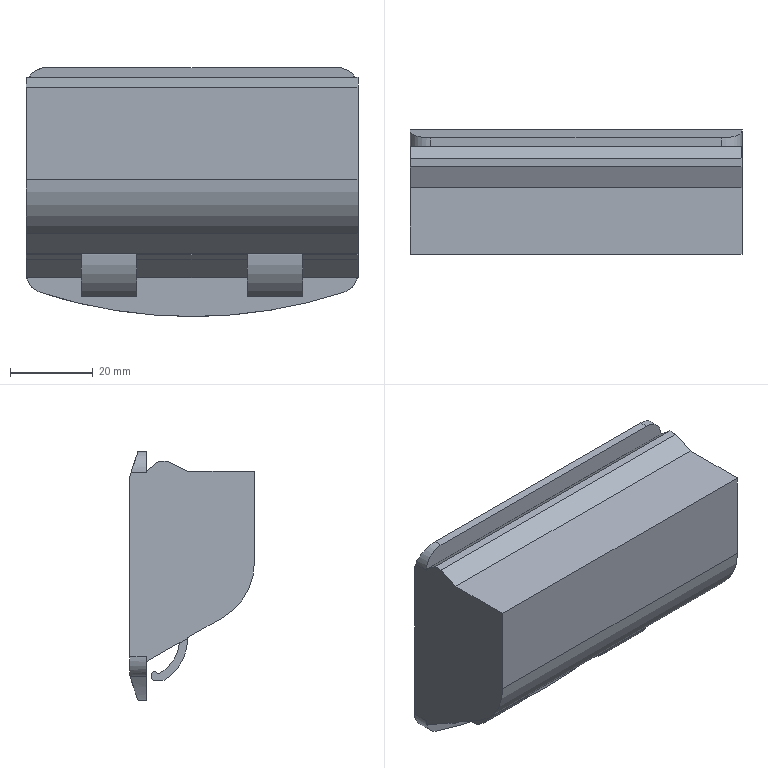Part | STEP file | ASND-0110-E63-HLTP01Grip handle UWAUNJ80 | 1 solid | 58 faces | box 80 x 30 x 60 mm | volume 51881 mm3 | plane 43 | cylinder 15 | commonest cylinder face diameters 6 x4 10 x4 30 x2 20 x1 24 x1 172.143 x1